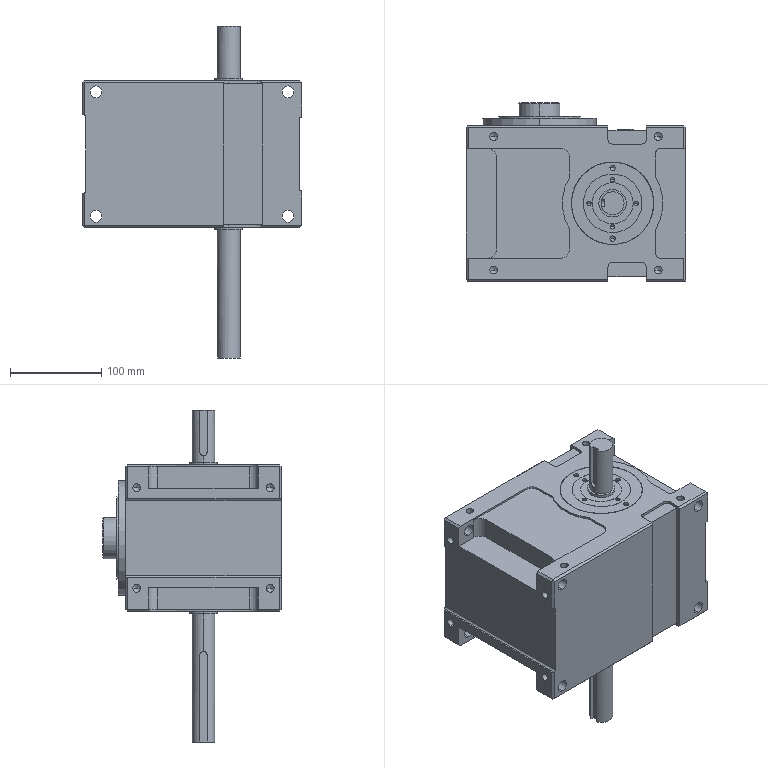Part | 3 solids | 583 faces | box 240 x 195 x 363 mm | volume 6118356 mm3 | plane 231 | cylinder 143 | spline 139 | cone 70 | commonest cylinder face diameters 8.5 x32 4.7 x16 13 x16 6.75 x12 10 x12 5.7 x8